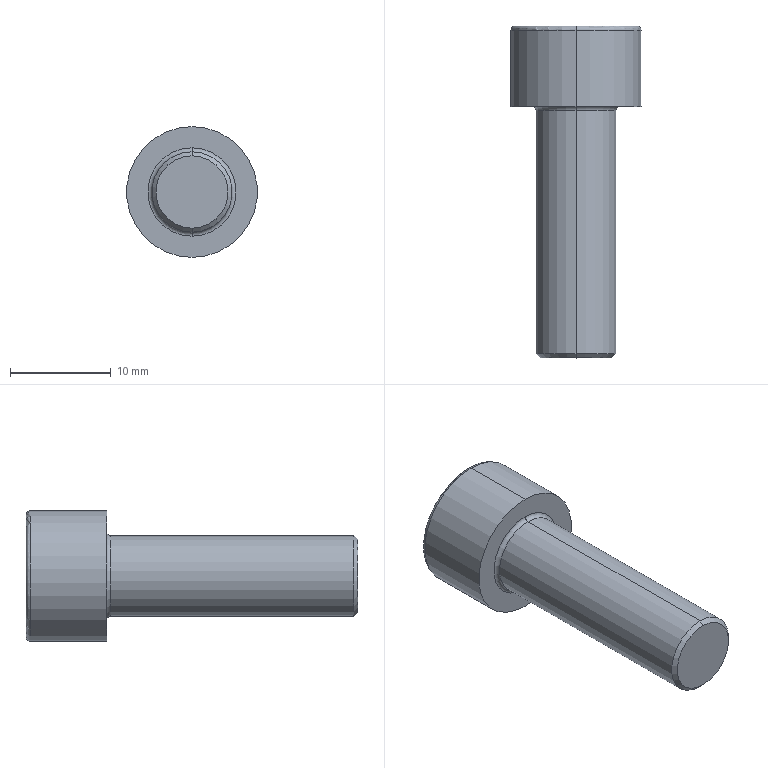Part | STEP file | 1 solid | 20 faces | box 13 x 33 x 13 mm | volume 2191 mm3 | plane 10 | torus 4 | cylinder 4 | cone 2 | commonest cylinder face diameters 8 x2 13 x2
STEP:
#1=CARTESIAN_POINT('',(0.,-25.,-3.6));
#2=VERTEX_POINT('',#1);
#3=CARTESIAN_POINT('',(0.,-25.,3.6));
#4=VERTEX_POINT('',#3);
#5=CARTESIAN_POINT('',(0.,-25.,0.));
#6=DIRECTION('',(0.,-1.,0.));
#7=DIRECTION('',(0.,0.,-1.));
#8=AXIS2_PLACEMENT_3D('',#5,#6,#7);
#9=CIRCLE('',#8,3.6);
#10=EDGE_CURVE('',#2,#4,#9,.T.);
#11=ORIENTED_EDGE('',*,*,#10,.F.);
#12=CARTESIAN_POINT('',(0.,-24.6,-4.));
#13=VERTEX_POINT('',#12);
#14=CARTESIAN_POINT('',(0.,-25.,-3.6));
#15=DIRECTION('',(0.,0.7071,-0.7071));
#16=VECTOR('',#15,1000.);
#17=LINE('',#14,#16);
#18=EDGE_CURVE('',#2,#13,#17,.T.);
#19=ORIENTED_EDGE('',*,*,#18,.T.);
#20=CARTESIAN_POINT('',(0.,-24.6,4.));
#21=VERTEX_POINT('',#20);
#22=CARTESIAN_POINT('',(0.,-24.6,0.));
#23=DIRECTION('',(0.,1.,0.));
#24=DIRECTION('',(0.,0.,-1.));
#25=AXIS2_PLACEMENT_3D('',#22,#23,#24);
#26=CIRCLE('',#25,4.);
#27=EDGE_CURVE('',#21,#13,#26,.T.);
#28=ORIENTED_EDGE('',*,*,#27,.F.);
#29=CARTESIAN_POINT('',(0.,-25.,3.6));
#30=DIRECTION('',(0.,0.7071,0.7071));
#31=VECTOR('',#30,1000.);
#32=LINE('',#29,#31);
#33=EDGE_CURVE('',#4,#21,#32,.T.);
#34=ORIENTED_EDGE('',*,*,#33,.F.);
#35=EDGE_LOOP('',(#11,#19,#28,#34));
#36=FACE_OUTER_BOUND('',#35,.T.);
#37=CARTESIAN_POINT('',(0.,-25.,0.));
#38=DIRECTION('',(0.,1.,0.));
#39=DIRECTION('',(0.,0.,1.));
#40=AXIS2_PLACEMENT_3D('',#37,#38,#39);
#41=CONICAL_SURFACE('',#40,3.6,0.7854);
#42=ADVANCED_FACE('',(#36),#41,.T.);
#43=CARTESIAN_POINT('',(0.,7.6,-6.5));
#44=VERTEX_POINT('',#43);
#45=CARTESIAN_POINT('',(0.,7.6,6.5));
#46=VERTEX_POINT('',#45);
#47=CARTESIAN_POINT('',(0.,7.6,0.));
#48=DIRECTION('',(0.,-1.,0.));
#49=DIRECTION('',(0.,0.,1.));
#50=AXIS2_PLACEMENT_3D('',#47,#48,#49);
#51=CIRCLE('',#50,6.5);
#52=EDGE_CURVE('',#44,#46,#51,.T.);
#53=ORIENTED_EDGE('',*,*,#52,.F.);
#54=CARTESIAN_POINT('',(0.,8.,-6.1));
#55=VERTEX_POINT('',#54);
#56=CARTESIAN_POINT('',(0.,7.6,-6.1));
#57=DIRECTION('',(1.,0.,0.));
#58=DIRECTION('',(0.,0.,-1.));
#59=AXIS2_PLACEMENT_3D('',#56,#57,#58);
#60=CIRCLE('',#59,0.4);
#61=EDGE_CURVE('',#44,#55,#60,.T.);
#62=ORIENTED_EDGE('',*,*,#61,.T.);
#63=CARTESIAN_POINT('',(0.,8.,6.1));
#64=VERTEX_POINT('',#63);
#65=CARTESIAN_POINT('',(0.,8.,0.));
#66=DIRECTION('',(0.,1.,0.));
#67=DIRECTION('',(0.,0.,1.));
#68=AXIS2_PLACEMENT_3D('',#65,#66,#67);
#69=CIRCLE('',#68,6.1);
#70=EDGE_CURVE('',#64,#55,#69,.T.);
#71=ORIENTED_EDGE('',*,*,#70,.F.);
#72=CARTESIAN_POINT('',(0.,7.6,6.1));
#73=DIRECTION('',(-1.,0.,0.));
#74=DIRECTION('',(0.,0.,1.));
#75=AXIS2_PLACEMENT_3D('',#72,#73,#74);
#76=CIRCLE('',#75,0.4);
#77=EDGE_CURVE('',#46,#64,#76,.T.);
#78=ORIENTED_EDGE('',*,*,#77,.F.);
#79=EDGE_LOOP('',(#53,#62,#71,#78));
#80=FACE_OUTER_BOUND('',#79,.T.);
#81=CARTESIAN_POINT('',(0.,7.6,0.));
#82=DIRECTION('',(0.,1.,0.));
#83=DIRECTION('',(0.,0.,1.));
#84=AXIS2_PLACEMENT_3D('',#81,#82,#83);
#85=TOROIDAL_SURFACE('',#84,6.1,0.4);
#86=ADVANCED_FACE('',(#80),#85,.T.);
#87=CARTESIAN_POINT('',(0.,-0.4,4.));
#88=VERTEX_POINT('',#87);
#89=CARTESIAN_POINT('',(0.,-0.4,-4.));
#90=VERTEX_POINT('',#89);
#91=CARTESIAN_POINT('',(0.,-0.4,0.));
#92=DIRECTION('',(0.,-1.,0.));
#93=DIRECTION('',(0.,0.,-1.));
#94=AXIS2_PLACEMENT_3D('',#91,#92,#93);
#95=CIRCLE('',#94,4.);
#96=EDGE_CURVE('',#88,#90,#95,.T.);
#97=ORIENTED_EDGE('',*,*,#96,.F.);
#98=CARTESIAN_POINT('',(0.,0.,4.4));
#99=VERTEX_POINT('',#98);
#100=CARTESIAN_POINT('',(0.,-0.4,4.4));
#101=DIRECTION('',(1.,0.,0.));
#102=DIRECTION('',(0.,0.,-1.));
#103=AXIS2_PLACEMENT_3D('',#100,#101,#102);
#104=CIRCLE('',#103,0.4);
#105=EDGE_CURVE('',#88,#99,#104,.T.);
#106=ORIENTED_EDGE('',*,*,#105,.T.);
#107=CARTESIAN_POINT('',(0.,0.,-4.4));
#108=VERTEX_POINT('',#107);
#109=CARTESIAN_POINT('',(0.,0.,0.));
#110=DIRECTION('',(0.,1.,0.));
#111=DIRECTION('',(0.,0.,-1.));
#112=AXIS2_PLACEMENT_3D('',#109,#110,#111);
#113=CIRCLE('',#112,4.4);
#114=EDGE_CURVE('',#108,#99,#113,.T.);
#115=ORIENTED_EDGE('',*,*,#114,.F.);
#116=CARTESIAN_POINT('',(0.,-0.4,-4.4));
#117=DIRECTION('',(-1.,0.,0.));
#118=DIRECTION('',(0.,0.,1.));
#119=AXIS2_PLACEMENT_3D('',#116,#117,#118);
#120=CIRCLE('',#119,0.4);
#121=EDGE_CURVE('',#90,#108,#120,.T.);
#122=ORIENTED_EDGE('',*,*,#121,.F.);
#123=EDGE_LOOP('',(#97,#106,#115,#122));
#124=FACE_OUTER_BOUND('',#123,.T.);
#125=CARTESIAN_POINT('',(0.,-0.4,0.));
#126=DIRECTION('',(0.,-1.,0.));
#127=DIRECTION('',(0.,0.,-1.));
#128=AXIS2_PLACEMENT_3D('',#125,#126,#127);
#129=TOROIDAL_SURFACE('',#128,4.4,0.4);
#130=ADVANCED_FACE('',(#124),#129,.F.);
#131=CARTESIAN_POINT('',(0.,-0.4,0.));
#132=DIRECTION('',(0.,-1.,0.));
#133=DIRECTION('',(0.,0.,-1.));
#134=AXIS2_PLACEMENT_3D('',#131,#132,#133);
#135=CIRCLE('',#134,4.);
#136=EDGE_CURVE('',#90,#88,#135,.T.);
#137=ORIENTED_EDGE('',*,*,#136,.T.);
#138=CARTESIAN_POINT('',(0.,0.,4.));
#139=DIRECTION('',(0.,-1.,0.));
#140=VECTOR('',#139,1000.);
#141=LINE('',#138,#140);
#142=EDGE_CURVE('',#88,#21,#141,.T.);
#143=ORIENTED_EDGE('',*,*,#142,.T.);
#144=ORIENTED_EDGE('',*,*,#27,.T.);
#145=CARTESIAN_POINT('',(0.,0.,-4.));
#146=DIRECTION('',(0.,-1.,0.));
#147=VECTOR('',#146,1000.);
#148=LINE('',#145,#147);
#149=EDGE_CURVE('',#90,#13,#148,.T.);
#150=ORIENTED_EDGE('',*,*,#149,.F.);
#151=EDGE_LOOP('',(#137,#143,#144,#150));
#152=FACE_OUTER_BOUND('',#151,.T.);
#153=CARTESIAN_POINT('',(0.,0.,0.));
#154=DIRECTION('',(0.,-1.,0.));
#155=DIRECTION('',(0.,0.,-1.));
#156=AXIS2_PLACEMENT_3D('',#153,#154,#155);
#157=CYLINDRICAL_SURFACE('',#156,4.);
#158=ADVANCED_FACE('',(#152),#157,.T.);
#159=ORIENTED_EDGE('',*,*,#52,.T.);
#160=CARTESIAN_POINT('',(0.,0.,6.5));
#161=VERTEX_POINT('',#160);
#162=CARTESIAN_POINT('',(0.,0.,6.5));
#163=DIRECTION('',(0.,-1.,0.));
#164=VECTOR('',#163,1000.);
#165=LINE('',#162,#164);
#166=EDGE_CURVE('',#46,#161,#165,.T.);
#167=ORIENTED_EDGE('',*,*,#166,.T.);
#168=CARTESIAN_POINT('',(0.,0.,-6.5));
#169=VERTEX_POINT('',#168);
#170=CARTESIAN_POINT('',(0.,0.,0.));
#171=DIRECTION('',(0.,-1.,0.));
#172=DIRECTION('',(0.,0.,-1.));
#173=AXIS2_PLACEMENT_3D('',#170,#171,#172);
#174=CIRCLE('',#173,6.5);
#175=EDGE_CURVE('',#169,#161,#174,.T.);
#176=ORIENTED_EDGE('',*,*,#175,.F.);
#177=CARTESIAN_POINT('',(0.,0.,-6.5));
#178=DIRECTION('',(0.,-1.,0.));
#179=VECTOR('',#178,1000.);
#180=LINE('',#177,#179);
#181=EDGE_CURVE('',#44,#169,#180,.T.);
#182=ORIENTED_EDGE('',*,*,#181,.F.);
#183=EDGE_LOOP('',(#159,#167,#176,#182));
#184=FACE_OUTER_BOUND('',#183,.T.);
#185=CARTESIAN_POINT('',(0.,0.,0.));
#186=DIRECTION('',(0.,-1.,0.));
#187=DIRECTION('',(0.,0.,-1.));
#188=AXIS2_PLACEMENT_3D('',#185,#186,#187);
#189=CYLINDRICAL_SURFACE('',#188,6.5);
#190=ADVANCED_FACE('',(#184),#189,.T.);
#191=ORIENTED_EDGE('',*,*,#70,.T.);
#192=CARTESIAN_POINT('',(0.,8.,0.));
#193=DIRECTION('',(0.,1.,0.));
#194=DIRECTION('',(0.,0.,1.));
#195=AXIS2_PLACEMENT_3D('',#192,#193,#194);
#196=CIRCLE('',#195,6.1);
#197=EDGE_CURVE('',#55,#64,#196,.T.);
#198=ORIENTED_EDGE('',*,*,#197,.T.);
#199=EDGE_LOOP('',(#191,#198));
#200=FACE_OUTER_BOUND('',#199,.T.);
#201=CARTESIAN_POINT('',(0.,8.,-3.464));
#202=VERTEX_POINT('',#201);
#203=CARTESIAN_POINT('',(-3.,8.,-1.732));
#204=VERTEX_POINT('',#203);
#205=CARTESIAN_POINT('',(0.,8.,-3.464));
#206=DIRECTION('',(-0.866,0.,0.5));
#207=VECTOR('',#206,1000.);
#208=LINE('',#205,#207);
#209=EDGE_CURVE('',#202,#204,#208,.T.);
#210=ORIENTED_EDGE('',*,*,#209,.F.);
#211=CARTESIAN_POINT('',(3.,8.,-1.732));
#212=VERTEX_POINT('',#211);
#213=CARTESIAN_POINT('',(3.,8.,-1.732));
#214=DIRECTION('',(-0.866,0.,-0.5));
#215=VECTOR('',#214,1000.);
#216=LINE('',#213,#215);
#217=EDGE_CURVE('',#212,#202,#216,.T.);
#218=ORIENTED_EDGE('',*,*,#217,.F.);
#219=CARTESIAN_POINT('',(3.,8.,1.732));
#220=VERTEX_POINT('',#219);
#221=CARTESIAN_POINT('',(3.,8.,1.732));
#222=DIRECTION('',(0.,0.,-1.));
#223=VECTOR('',#222,1000.);
#224=LINE('',#221,#223);
#225=EDGE_CURVE('',#220,#212,#224,.T.);
#226=ORIENTED_EDGE('',*,*,#225,.F.);
#227=CARTESIAN_POINT('',(0.,8.,3.464));
#228=VERTEX_POINT('',#227);
#229=CARTESIAN_POINT('',(0.,8.,3.464));
#230=DIRECTION('',(0.866,0.,-0.5));
#231=VECTOR('',#230,1000.);
#232=LINE('',#229,#231);
#233=EDGE_CURVE('',#228,#220,#232,.T.);
#234=ORIENTED_EDGE('',*,*,#233,.F.);
#235=CARTESIAN_POINT('',(-3.,8.,1.732));
#236=VERTEX_POINT('',#235);
#237=CARTESIAN_POINT('',(-3.,8.,1.732));
#238=DIRECTION('',(0.866,0.,0.5));
#239=VECTOR('',#238,1000.);
#240=LINE('',#237,#239);
#241=EDGE_CURVE('',#236,#228,#240,.T.);
#242=ORIENTED_EDGE('',*,*,#241,.F.);
#243=CARTESIAN_POINT('',(-3.,8.,-1.732));
#244=DIRECTION('',(0.,0.,1.));
#245=VECTOR('',#244,1000.);
#246=LINE('',#243,#245);
#247=EDGE_CURVE('',#204,#236,#246,.T.);
#248=ORIENTED_EDGE('',*,*,#247,.F.);
#249=EDGE_LOOP('',(#210,#218,#226,#234,#242,#248));
#250=FACE_BOUND('',#249,.T.);
#251=CARTESIAN_POINT('',(0.,8.,0.));
#252=DIRECTION('',(0.,1.,0.));
#253=DIRECTION('',(0.,0.,1.));
#254=AXIS2_PLACEMENT_3D('',#251,#252,#253);
#255=PLANE('',#254);
#256=ADVANCED_FACE('',(#200,#250),#255,.T.);
#257=ORIENTED_EDGE('',*,*,#166,.F.);
#258=CARTESIAN_POINT('',(0.,7.6,0.));
#259=DIRECTION('',(0.,-1.,0.));
#260=DIRECTION('',(0.,0.,1.));
#261=AXIS2_PLACEMENT_3D('',#258,#259,#260);
#262=CIRCLE('',#261,6.5);
#263=EDGE_CURVE('',#46,#44,#262,.T.);
#264=ORIENTED_EDGE('',*,*,#263,.T.);
#265=ORIENTED_EDGE('',*,*,#181,.T.);
#266=CARTESIAN_POINT('',(0.,0.,0.));
#267=DIRECTION('',(0.,-1.,0.));
#268=DIRECTION('',(0.,0.,-1.));
#269=AXIS2_PLACEMENT_3D('',#266,#267,#268);
#270=CIRCLE('',#269,6.5);
#271=EDGE_CURVE('',#161,#169,#270,.T.);
#272=ORIENTED_EDGE('',*,*,#271,.F.);
#273=EDGE_LOOP('',(#257,#264,#265,#272));
#274=FACE_OUTER_BOUND('',#273,.T.);
#275=CARTESIAN_POINT('',(0.,0.,0.));
#276=DIRECTION('',(0.,-1.,0.));
#277=DIRECTION('',(0.,0.,-1.));
#278=AXIS2_PLACEMENT_3D('',#275,#276,#277);
#279=CYLINDRICAL_SURFACE('',#278,6.5);
#280=ADVANCED_FACE('',(#274),#279,.T.);
#281=ORIENTED_EDGE('',*,*,#114,.T.);
#282=CARTESIAN_POINT('',(0.,0.,0.));
#283=DIRECTION('',(0.,1.,0.));
#284=DIRECTION('',(0.,0.,-1.));
#285=AXIS2_PLACEMENT_3D('',#282,#283,#284);
#286=CIRCLE('',#285,4.4);
#287=EDGE_CURVE('',#99,#108,#286,.T.);
#288=ORIENTED_EDGE('',*,*,#287,.T.);
#289=EDGE_LOOP('',(#281,#288));
#290=FACE_BOUND('',#289,.T.);
#291=ORIENTED_EDGE('',*,*,#175,.T.);
#292=ORIENTED_EDGE('',*,*,#271,.T.);
#293=EDGE_LOOP('',(#291,#292));
#294=FACE_OUTER_BOUND('',#293,.T.);
#295=CARTESIAN_POINT('',(6.5,0.,0.));
#296=DIRECTION('',(0.,-1.,0.));
#297=DIRECTION('',(0.,0.,-1.));
#298=AXIS2_PLACEMENT_3D('',#295,#296,#297);
#299=PLANE('',#298);
#300=ADVANCED_FACE('',(#290,#294),#299,.T.);
#301=ORIENTED_EDGE('',*,*,#142,.F.);
#302=ORIENTED_EDGE('',*,*,#96,.T.);
#303=ORIENTED_EDGE('',*,*,#149,.T.);
#304=CARTESIAN_POINT('',(0.,-24.6,0.));
#305=DIRECTION('',(0.,1.,0.));
#306=DIRECTION('',(0.,0.,-1.));
#307=AXIS2_PLACEMENT_3D('',#304,#305,#306);
#308=CIRCLE('',#307,4.);
#309=EDGE_CURVE('',#13,#21,#308,.T.);
#310=ORIENTED_EDGE('',*,*,#309,.T.);
#311=EDGE_LOOP('',(#301,#302,#303,#310));
#312=FACE_OUTER_BOUND('',#311,.T.);
#313=CARTESIAN_POINT('',(0.,0.,0.));
#314=DIRECTION('',(0.,-1.,0.));
#315=DIRECTION('',(0.,0.,-1.));
#316=AXIS2_PLACEMENT_3D('',#313,#314,#315);
#317=CYLINDRICAL_SURFACE('',#316,4.);
#318=ADVANCED_FACE('',(#312),#317,.T.);
#319=CARTESIAN_POINT('',(0.,-25.,0.));
#320=DIRECTION('',(0.,-1.,0.));
#321=DIRECTION('',(0.,0.,-1.));
#322=AXIS2_PLACEMENT_3D('',#319,#320,#321);
#323=CIRCLE('',#322,3.6);
#324=EDGE_CURVE('',#4,#2,#323,.T.);
#325=ORIENTED_EDGE('',*,*,#324,.T.);
#326=ORIENTED_EDGE('',*,*,#10,.T.);
#327=EDGE_LOOP('',(#325,#326));
#328=FACE_OUTER_BOUND('',#327,.T.);
#329=CARTESIAN_POINT('',(4.,-25.,0.));
#330=DIRECTION('',(0.,-1.,0.));
#331=DIRECTION('',(0.,0.,-1.));
#332=AXIS2_PLACEMENT_3D('',#329,#330,#331);
#333=PLANE('',#332);
#334=ADVANCED_FACE('',(#328),#333,.T.);
#335=ORIENTED_EDGE('',*,*,#209,.T.);
#336=CARTESIAN_POINT('',(-3.,4.,-1.732));
#337=VERTEX_POINT('',#336);
#338=CARTESIAN_POINT('',(-3.,4.,-1.732));
#339=DIRECTION('',(0.,1.,0.));
#340=VECTOR('',#339,1000.);
#341=LINE('',#338,#340);
#342=EDGE_CURVE('',#337,#204,#341,.T.);
#343=ORIENTED_EDGE('',*,*,#342,.F.);
#344=CARTESIAN_POINT('',(0.,4.,-3.464));
#345=VERTEX_POINT('',#344);
#346=CARTESIAN_POINT('',(0.,4.,-3.464));
#347=DIRECTION('',(-0.866,0.,0.5));
#348=VECTOR('',#347,1000.);
#349=LINE('',#346,#348);
#350=EDGE_CURVE('',#345,#337,#349,.T.);
#351=ORIENTED_EDGE('',*,*,#350,.F.);
#352=CARTESIAN_POINT('',(0.,4.,-3.464));
#353=DIRECTION('',(0.,1.,0.));
#354=VECTOR('',#353,1000.);
#355=LINE('',#352,#354);
#356=EDGE_CURVE('',#345,#202,#355,.T.);
#357=ORIENTED_EDGE('',*,*,#356,.T.);
#358=EDGE_LOOP('',(#335,#343,#351,#357));
#359=FACE_OUTER_BOUND('',#358,.T.);
#360=CARTESIAN_POINT('',(0.,4.,-3.464));
#361=DIRECTION('',(-0.5,0.,-0.866));
#362=DIRECTION('',(-0.866,0.,0.5));
#363=AXIS2_PLACEMENT_3D('',#360,#361,#362);
#364=PLANE('',#363);
#365=ADVANCED_FACE('',(#359),#364,.F.);
#366=ORIENTED_EDGE('',*,*,#217,.T.);
#367=ORIENTED_EDGE('',*,*,#356,.F.);
#368=CARTESIAN_POINT('',(3.,4.,-1.732));
#369=VERTEX_POINT('',#368);
#370=CARTESIAN_POINT('',(3.,4.,-1.732));
#371=DIRECTION('',(-0.866,0.,-0.5));
#372=VECTOR('',#371,1000.);
#373=LINE('',#370,#372);
#374=EDGE_CURVE('',#369,#345,#373,.T.);
#375=ORIENTED_EDGE('',*,*,#374,.F.);
#376=CARTESIAN_POINT('',(3.,4.,-1.732));
#377=DIRECTION('',(0.,1.,0.));
#378=VECTOR('',#377,1000.);
#379=LINE('',#376,#378);
#380=EDGE_CURVE('',#369,#212,#379,.T.);
#381=ORIENTED_EDGE('',*,*,#380,.T.);
#382=EDGE_LOOP('',(#366,#367,#375,#381));
#383=FACE_OUTER_BOUND('',#382,.T.);
#384=CARTESIAN_POINT('',(3.,4.,-1.732));
#385=DIRECTION('',(0.5,0.,-0.866));
#386=DIRECTION('',(-0.866,0.,-0.5));
#387=AXIS2_PLACEMENT_3D('',#384,#385,#386);
#388=PLANE('',#387);
#389=ADVANCED_FACE('',(#383),#388,.F.);
#390=ORIENTED_EDGE('',*,*,#225,.T.);
#391=ORIENTED_EDGE('',*,*,#380,.F.);
#392=CARTESIAN_POINT('',(3.,4.,1.732));
#393=VERTEX_POINT('',#392);
#394=CARTESIAN_POINT('',(3.,4.,1.732));
#395=DIRECTION('',(0.,0.,-1.));
#396=VECTOR('',#395,1000.);
#397=LINE('',#394,#396);
#398=EDGE_CURVE('',#393,#369,#397,.T.);
#399=ORIENTED_EDGE('',*,*,#398,.F.);
#400=CARTESIAN_POINT('',(3.,4.,1.732));
#401=DIRECTION('',(0.,1.,0.));
#402=VECTOR('',#401,1000.);
#403=LINE('',#400,#402);
#404=EDGE_CURVE('',#393,#220,#403,.T.);
#405=ORIENTED_EDGE('',*,*,#404,.T.);
#406=EDGE_LOOP('',(#390,#391,#399,#405));
#407=FACE_OUTER_BOUND('',#406,.T.);
#408=CARTESIAN_POINT('',(3.,4.,1.732));
#409=DIRECTION('',(1.,0.,0.));
#410=DIRECTION('',(0.,0.,-1.));
#411=AXIS2_PLACEMENT_3D('',#408,#409,#410);
#412=PLANE('',#411);
#413=ADVANCED_FACE('',(#407),#412,.F.);
#414=ORIENTED_EDGE('',*,*,#233,.T.);
#415=ORIENTED_EDGE('',*,*,#404,.F.);
#416=CARTESIAN_POINT('',(0.,4.,3.464));
#417=VERTEX_POINT('',#416);
#418=CARTESIAN_POINT('',(0.,4.,3.464));
#419=DIRECTION('',(0.866,0.,-0.5));
#420=VECTOR('',#419,1000.);
#421=LINE('',#418,#420);
#422=EDGE_CURVE('',#417,#393,#421,.T.);
#423=ORIENTED_EDGE('',*,*,#422,.F.);
#424=CARTESIAN_POINT('',(0.,4.,3.464));
#425=DIRECTION('',(0.,1.,0.));
#426=VECTOR('',#425,1000.);
#427=LINE('',#424,#426);
#428=EDGE_CURVE('',#417,#228,#427,.T.);
#429=ORIENTED_EDGE('',*,*,#428,.T.);
#430=EDGE_LOOP('',(#414,#415,#423,#429));
#431=FACE_OUTER_BOUND('',#430,.T.);
#432=CARTESIAN_POINT('',(0.,4.,3.464));
#433=DIRECTION('',(0.5,0.,0.866));
#434=DIRECTION('',(0.866,0.,-0.5));
#435=AXIS2_PLACEMENT_3D('',#432,#433,#434);
#436=PLANE('',#435);
#437=ADVANCED_FACE('',(#431),#436,.F.);
#438=ORIENTED_EDGE('',*,*,#241,.T.);
#439=ORIENTED_EDGE('',*,*,#428,.F.);
#440=CARTESIAN_POINT('',(-3.,4.,1.732));
#441=VERTEX_POINT('',#440);
#442=CARTESIAN_POINT('',(-3.,4.,1.732));
#443=DIRECTION('',(0.866,0.,0.5));
#444=VECTOR('',#443,1000.);
#445=LINE('',#442,#444);
#446=EDGE_CURVE('',#441,#417,#445,.T.);
#447=ORIENTED_EDGE('',*,*,#446,.F.);
#448=CARTESIAN_POINT('',(-3.,4.,1.732));
#449=DIRECTION('',(0.,1.,0.));
#450=VECTOR('',#449,1000.);
#451=LINE('',#448,#450);
#452=EDGE_CURVE('',#441,#236,#451,.T.);
#453=ORIENTED_EDGE('',*,*,#452,.T.);
#454=EDGE_LOOP('',(#438,#439,#447,#453));
#455=FACE_OUTER_BOUND('',#454,.T.);
#456=CARTESIAN_POINT('',(-3.,4.,1.732));
#457=DIRECTION('',(-0.5,0.,0.866));
#458=DIRECTION('',(0.866,0.,0.5));
#459=AXIS2_PLACEMENT_3D('',#456,#457,#458);
#460=PLANE('',#459);
#461=ADVANCED_FACE('',(#455),#460,.F.);
#462=ORIENTED_EDGE('',*,*,#247,.T.);
#463=ORIENTED_EDGE('',*,*,#452,.F.);
#464=CARTESIAN_POINT('',(-3.,4.,-1.732));
#465=DIRECTION('',(0.,0.,1.));
#466=VECTOR('',#465,1000.);
#467=LINE('',#464,#466);
#468=EDGE_CURVE('',#337,#441,#467,.T.);
#469=ORIENTED_EDGE('',*,*,#468,.F.);
#470=ORIENTED_EDGE('',*,*,#342,.T.);
#471=EDGE_LOOP('',(#462,#463,#469,#470));
#472=FACE_OUTER_BOUND('',#471,.T.);
#473=CARTESIAN_POINT('',(-3.,4.,-1.732));
#474=DIRECTION('',(-1.,0.,0.));
#475=DIRECTION('',(0.,0.,1.));
#476=AXIS2_PLACEMENT_3D('',#473,#474,#475);
#477=PLANE('',#476);
#478=ADVANCED_FACE('',(#472),#477,.F.);
#479=ORIENTED_EDGE('',*,*,#350,.T.);
#480=ORIENTED_EDGE('',*,*,#468,.T.);
#481=ORIENTED_EDGE('',*,*,#446,.T.);
#482=ORIENTED_EDGE('',*,*,#422,.T.);
#483=ORIENTED_EDGE('',*,*,#398,.T.);
#484=ORIENTED_EDGE('',*,*,#374,.T.);
#485=EDGE_LOOP('',(#479,#480,#481,#482,#483,#484));
#486=FACE_OUTER_BOUND('',#485,.T.);
#487=CARTESIAN_POINT('',(0.,4.,0.));
#488=DIRECTION('',(0.,1.,0.));
#489=DIRECTION('',(0.,0.,1.));
#490=AXIS2_PLACEMENT_3D('',#487,#488,#489);
#491=PLANE('',#490);
#492=ADVANCED_FACE('',(#486),#491,.T.);
#493=ORIENTED_EDGE('',*,*,#105,.F.);
#494=ORIENTED_EDGE('',*,*,#136,.F.);
#495=ORIENTED_EDGE('',*,*,#121,.T.);
#496=ORIENTED_EDGE('',*,*,#287,.F.);
#497=EDGE_LOOP('',(#493,#494,#495,#496));
#498=FACE_OUTER_BOUND('',#497,.T.);
#499=CARTESIAN_POINT('',(0.,-0.4,0.));
#500=DIRECTION('',(0.,-1.,0.));
#501=DIRECTION('',(0.,0.,-1.));
#502=AXIS2_PLACEMENT_3D('',#499,#500,#501);
#503=TOROIDAL_SURFACE('',#502,4.4,0.4);
#504=ADVANCED_FACE('',(#498),#503,.F.);
#505=ORIENTED_EDGE('',*,*,#61,.F.);
#506=ORIENTED_EDGE('',*,*,#263,.F.);
#507=ORIENTED_EDGE('',*,*,#77,.T.);
#508=ORIENTED_EDGE('',*,*,#197,.F.);
#509=EDGE_LOOP('',(#505,#506,#507,#508));
#510=FACE_OUTER_BOUND('',#509,.T.);
#511=CARTESIAN_POINT('',(0.,7.6,0.));
#512=DIRECTION('',(0.,1.,0.));
#513=DIRECTION('',(0.,0.,1.));
#514=AXIS2_PLACEMENT_3D('',#511,#512,#513);
#515=TOROIDAL_SURFACE('',#514,6.1,0.4);
#516=ADVANCED_FACE('',(#510),#515,.T.);
#517=ORIENTED_EDGE('',*,*,#18,.F.);
#518=ORIENTED_EDGE('',*,*,#324,.F.);
#519=ORIENTED_EDGE('',*,*,#33,.T.);
#520=ORIENTED_EDGE('',*,*,#309,.F.);
#521=EDGE_LOOP('',(#517,#518,#519,#520));
#522=FACE_OUTER_BOUND('',#521,.T.);
#523=CARTESIAN_POINT('',(0.,-25.,0.));
#524=DIRECTION('',(0.,1.,0.));
#525=DIRECTION('',(0.,0.,1.));
#526=AXIS2_PLACEMENT_3D('',#523,#524,#525);
#527=CONICAL_SURFACE('',#526,3.6,0.7854);
#528=ADVANCED_FACE('',(#522),#527,.T.);
#529=CLOSED_SHELL('',(#42,#86,#130,#158,#190,#256,#280,#300,#318,#334,#365,#389,#413,#437,#461,#478,#492,#504,#516,#528));
#530=MANIFOLD_SOLID_BREP('',#529);
#531=CARTESIAN_POINT('',(0.,0.,0.));
#532=DIRECTION('',(0.,0.,1.));
#533=DIRECTION('',(1.,0.,0.));
#534=AXIS2_PLACEMENT_3D('',#531,#532,#533);
#535=(LENGTH_UNIT()NAMED_UNIT(*)SI_UNIT(.MILLI.,.METRE.));
#536=UNCERTAINTY_MEASURE_WITH_UNIT(LENGTH_MEASURE(0.00001),#535,'','');
#537=(NAMED_UNIT(*)PLANE_ANGLE_UNIT()SI_UNIT($,.RADIAN.));
#538=(NAMED_UNIT(*)SI_UNIT($,.STERADIAN.)SOLID_ANGLE_UNIT());
#539=(GEOMETRIC_REPRESENTATION_CONTEXT(3)GLOBAL_UNCERTAINTY_ASSIGNED_CONTEXT((#536))GLOBAL_UNIT_ASSIGNED_CONTEXT((#535,#537,#538))REPRESENTATION_CONTEXT('',''));
#540=ADVANCED_BREP_SHAPE_REPRESENTATION('',(#530,#534),#539);